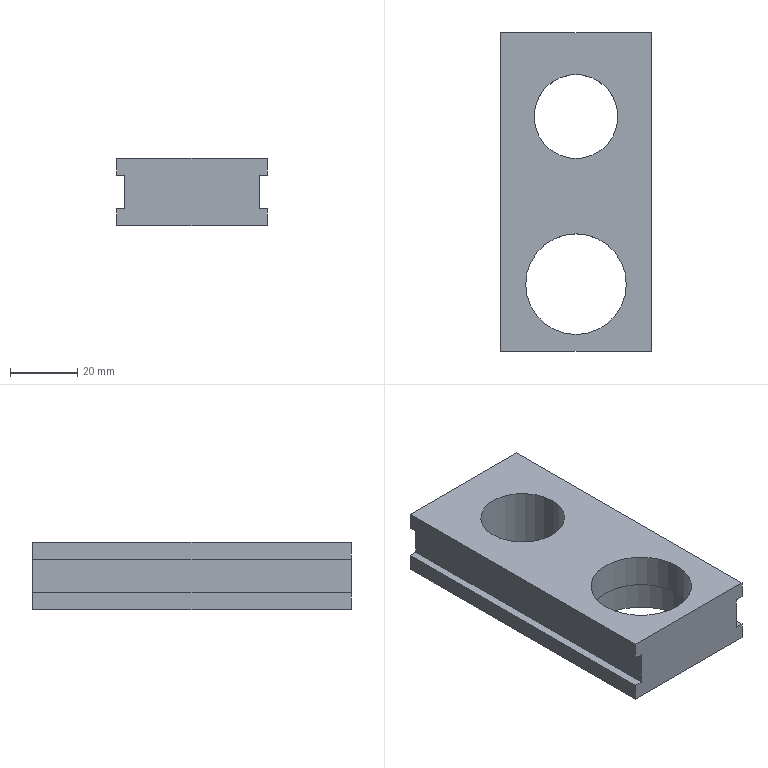Part | STEP file | A14-014 | 1 solid | 24 faces | box 45 x 95 x 20 mm | volume 53108 mm3 | plane 16 | cylinder 8 | commonest cylinder face diameters 17 x2 25 x2 30 x2 35 x2